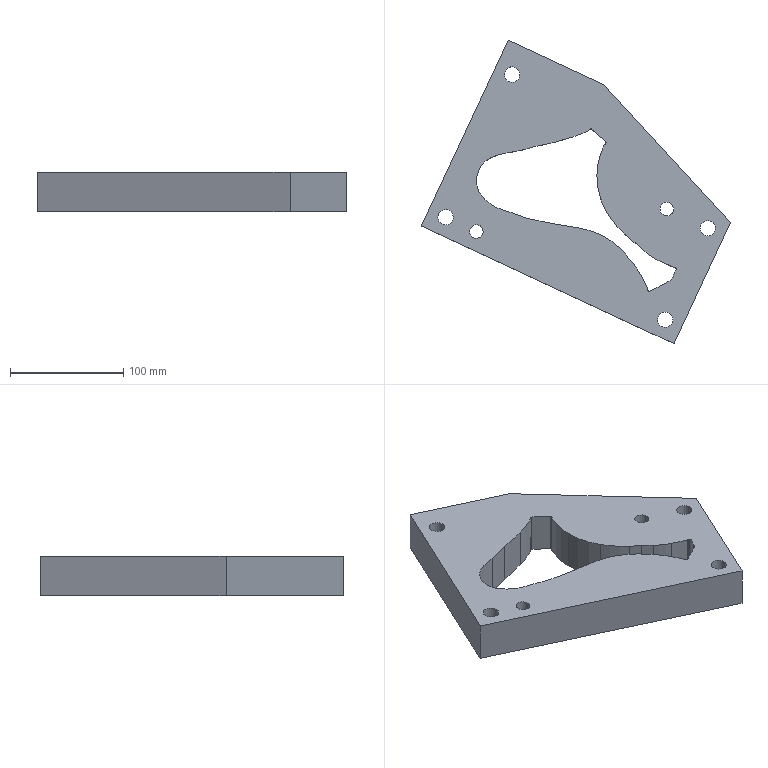Part | NX | features 7 2 | 1 solid | 79 faces | box 272.821 x 268.006 x 35 mm | volume 1037215 mm3 | cylinder 54 | plane 23 | cone 2 | commonest cylinder face diameters 2 x12 13.5 x4 20 x4 5.199 x2 10 x2 12.001 x2